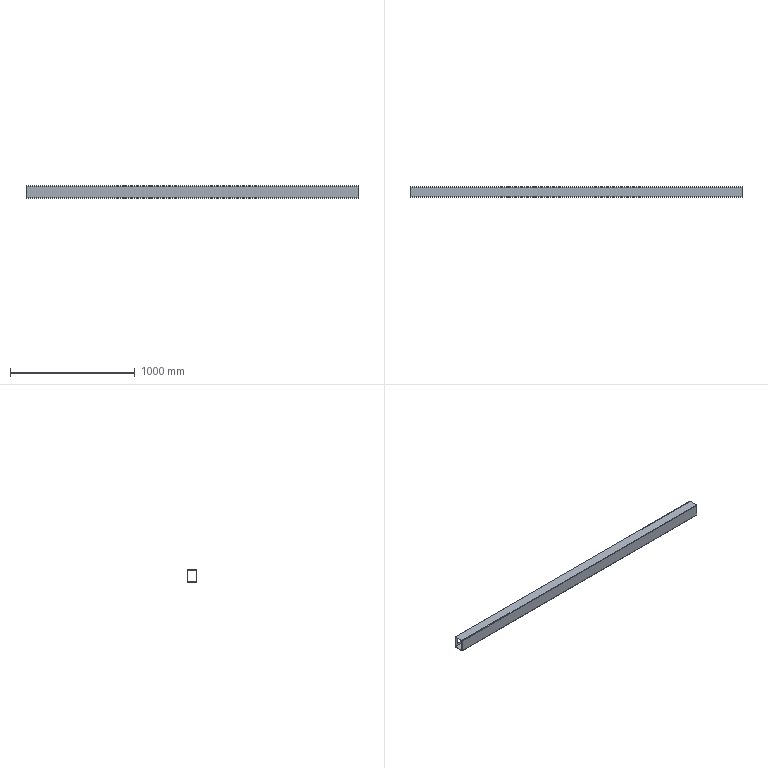Part | SolidWorks | features BaseBody 1 | 1 solid | 34 faces | box 2660 x 80 x 100 mm | volume 2713722 mm3 | plane 18 | cylinder 16 | commonest cylinder face diameters 8 x8 1 x4 7 x4
STEP:
#1=CARTESIAN_POINT('',(-1330.,40.,-46.5));
#2=VERTEX_POINT('',#1);
#3=CARTESIAN_POINT('',(-1330.,40.,46.5));
#4=VERTEX_POINT('',#3);
#5=CARTESIAN_POINT('',(-1330.,40.,46.5));
#6=DIRECTION('',(0.,0.,1.));
#7=VECTOR('',#6,1000.);
#8=LINE('',#5,#7);
#9=EDGE_CURVE('',#2,#4,#8,.T.);
#10=ORIENTED_EDGE('',*,*,#9,.T.);
#11=CARTESIAN_POINT('',(1330.,40.,46.5));
#12=VERTEX_POINT('',#11);
#13=CARTESIAN_POINT('',(1330.,40.,46.5));
#14=DIRECTION('',(-1.,0.,0.));
#15=VECTOR('',#14,1000.);
#16=LINE('',#13,#15);
#17=EDGE_CURVE('',#12,#4,#16,.T.);
#18=ORIENTED_EDGE('',*,*,#17,.F.);
#19=CARTESIAN_POINT('',(1330.,40.,-46.5));
#20=VERTEX_POINT('',#19);
#21=CARTESIAN_POINT('',(1330.,40.,46.5));
#22=DIRECTION('',(0.,0.,1.));
#23=VECTOR('',#22,1000.);
#24=LINE('',#21,#23);
#25=EDGE_CURVE('',#20,#12,#24,.T.);
#26=ORIENTED_EDGE('',*,*,#25,.F.);
#27=CARTESIAN_POINT('',(1330.,40.,-46.5));
#28=DIRECTION('',(-1.,0.,0.));
#29=VECTOR('',#28,1000.);
#30=LINE('',#27,#29);
#31=EDGE_CURVE('',#20,#2,#30,.T.);
#32=ORIENTED_EDGE('',*,*,#31,.T.);
#33=EDGE_LOOP('',(#10,#18,#26,#32));
#34=FACE_OUTER_BOUND('',#33,.T.);
#35=CARTESIAN_POINT('',(-1209.,40.,-30.));
#36=VERTEX_POINT('',#35);
#37=CARTESIAN_POINT('',(-1301.,40.,-30.));
#38=VERTEX_POINT('',#37);
#39=CARTESIAN_POINT('',(-1301.,40.,-30.));
#40=DIRECTION('',(-1.,0.,0.));
#41=VECTOR('',#40,1000.);
#42=LINE('',#39,#41);
#43=EDGE_CURVE('',#36,#38,#42,.T.);
#44=ORIENTED_EDGE('',*,*,#43,.F.);
#45=CARTESIAN_POINT('',(-1205.,40.,-26.));
#46=VERTEX_POINT('',#45);
#47=CARTESIAN_POINT('',(-1209.,40.,-26.));
#48=DIRECTION('',(0.,1.,0.));
#49=DIRECTION('',(0.,0.,1.));
#50=AXIS2_PLACEMENT_3D('',#47,#48,#49);
#51=CIRCLE('',#50,4.);
#52=EDGE_CURVE('',#46,#36,#51,.T.);
#53=ORIENTED_EDGE('',*,*,#52,.F.);
#54=CARTESIAN_POINT('',(-1205.,40.,26.));
#55=VERTEX_POINT('',#54);
#56=CARTESIAN_POINT('',(-1205.,40.,-26.));
#57=DIRECTION('',(0.,0.,-1.));
#58=VECTOR('',#57,1000.);
#59=LINE('',#56,#58);
#60=EDGE_CURVE('',#55,#46,#59,.T.);
#61=ORIENTED_EDGE('',*,*,#60,.F.);
#62=CARTESIAN_POINT('',(-1209.,40.,30.));
#63=VERTEX_POINT('',#62);
#64=CARTESIAN_POINT('',(-1209.,40.,26.));
#65=DIRECTION('',(0.,1.,0.));
#66=DIRECTION('',(0.,0.,1.));
#67=AXIS2_PLACEMENT_3D('',#64,#65,#66);
#68=CIRCLE('',#67,4.);
#69=EDGE_CURVE('',#63,#55,#68,.T.);
#70=ORIENTED_EDGE('',*,*,#69,.F.);
#71=CARTESIAN_POINT('',(-1301.,40.,30.));
#72=VERTEX_POINT('',#71);
#73=CARTESIAN_POINT('',(-1301.,40.,30.));
#74=DIRECTION('',(1.,0.,0.));
#75=VECTOR('',#74,1000.);
#76=LINE('',#73,#75);
#77=EDGE_CURVE('',#72,#63,#76,.T.);
#78=ORIENTED_EDGE('',*,*,#77,.F.);
#79=CARTESIAN_POINT('',(-1305.,40.,26.));
#80=VERTEX_POINT('',#79);
#81=CARTESIAN_POINT('',(-1301.,40.,26.));
#82=DIRECTION('',(0.,1.,0.));
#83=DIRECTION('',(0.,0.,1.));
#84=AXIS2_PLACEMENT_3D('',#81,#82,#83);
#85=CIRCLE('',#84,4.);
#86=EDGE_CURVE('',#80,#72,#85,.T.);
#87=ORIENTED_EDGE('',*,*,#86,.F.);
#88=CARTESIAN_POINT('',(-1305.,40.,-26.));
#89=VERTEX_POINT('',#88);
#90=CARTESIAN_POINT('',(-1305.,40.,-26.));
#91=DIRECTION('',(0.,0.,1.));
#92=VECTOR('',#91,1000.);
#93=LINE('',#90,#92);
#94=EDGE_CURVE('',#89,#80,#93,.T.);
#95=ORIENTED_EDGE('',*,*,#94,.F.);
#96=CARTESIAN_POINT('',(-1301.,40.,-26.));
#97=DIRECTION('',(0.,1.,0.));
#98=DIRECTION('',(0.,0.,1.));
#99=AXIS2_PLACEMENT_3D('',#96,#97,#98);
#100=CIRCLE('',#99,4.);
#101=EDGE_CURVE('',#38,#89,#100,.T.);
#102=ORIENTED_EDGE('',*,*,#101,.F.);
#103=EDGE_LOOP('',(#44,#53,#61,#70,#78,#87,#95,#102));
#104=FACE_BOUND('',#103,.T.);
#105=CARTESIAN_POINT('',(1205.,40.,-26.));
#106=VERTEX_POINT('',#105);
#107=CARTESIAN_POINT('',(1209.,40.,-30.));
#108=VERTEX_POINT('',#107);
#109=CARTESIAN_POINT('',(1209.,40.,-26.));
#110=DIRECTION('',(0.,-1.,0.));
#111=DIRECTION('',(0.,0.,1.));
#112=AXIS2_PLACEMENT_3D('',#109,#110,#111);
#113=CIRCLE('',#112,4.);
#114=EDGE_CURVE('',#106,#108,#113,.T.);
#115=ORIENTED_EDGE('',*,*,#114,.T.);
#116=CARTESIAN_POINT('',(1301.,40.,-30.));
#117=VERTEX_POINT('',#116);
#118=CARTESIAN_POINT('',(1330.,40.,-30.));
#119=DIRECTION('',(1.,0.,0.));
#120=VECTOR('',#119,1000.);
#121=LINE('',#118,#120);
#122=EDGE_CURVE('',#108,#117,#121,.T.);
#123=ORIENTED_EDGE('',*,*,#122,.T.);
#124=CARTESIAN_POINT('',(1305.,40.,-26.));
#125=VERTEX_POINT('',#124);
#126=CARTESIAN_POINT('',(1301.,40.,-26.));
#127=DIRECTION('',(0.,-1.,0.));
#128=DIRECTION('',(0.,0.,1.));
#129=AXIS2_PLACEMENT_3D('',#126,#127,#128);
#130=CIRCLE('',#129,4.);
#131=EDGE_CURVE('',#117,#125,#130,.T.);
#132=ORIENTED_EDGE('',*,*,#131,.T.);
#133=CARTESIAN_POINT('',(1305.,40.,26.));
#134=VERTEX_POINT('',#133);
#135=CARTESIAN_POINT('',(1305.,40.,46.5));
#136=DIRECTION('',(0.,0.,1.));
#137=VECTOR('',#136,1000.);
#138=LINE('',#135,#137);
#139=EDGE_CURVE('',#125,#134,#138,.T.);
#140=ORIENTED_EDGE('',*,*,#139,.T.);
#141=CARTESIAN_POINT('',(1301.,40.,30.));
#142=VERTEX_POINT('',#141);
#143=CARTESIAN_POINT('',(1301.,40.,26.));
#144=DIRECTION('',(0.,-1.,0.));
#145=DIRECTION('',(0.,0.,1.));
#146=AXIS2_PLACEMENT_3D('',#143,#144,#145);
#147=CIRCLE('',#146,4.);
#148=EDGE_CURVE('',#134,#142,#147,.T.);
#149=ORIENTED_EDGE('',*,*,#148,.T.);
#150=CARTESIAN_POINT('',(1209.,40.,30.));
#151=VERTEX_POINT('',#150);
#152=CARTESIAN_POINT('',(1330.,40.,30.));
#153=DIRECTION('',(-1.,0.,0.));
#154=VECTOR('',#153,1000.);
#155=LINE('',#152,#154);
#156=EDGE_CURVE('',#142,#151,#155,.T.);
#157=ORIENTED_EDGE('',*,*,#156,.T.);
#158=CARTESIAN_POINT('',(1205.,40.,26.));
#159=VERTEX_POINT('',#158);
#160=CARTESIAN_POINT('',(1209.,40.,26.));
#161=DIRECTION('',(0.,-1.,0.));
#162=DIRECTION('',(0.,0.,1.));
#163=AXIS2_PLACEMENT_3D('',#160,#161,#162);
#164=CIRCLE('',#163,4.);
#165=EDGE_CURVE('',#151,#159,#164,.T.);
#166=ORIENTED_EDGE('',*,*,#165,.T.);
#167=CARTESIAN_POINT('',(1205.,40.,46.5));
#168=DIRECTION('',(0.,0.,-1.));
#169=VECTOR('',#168,1000.);
#170=LINE('',#167,#169);
#171=EDGE_CURVE('',#159,#106,#170,.T.);
#172=ORIENTED_EDGE('',*,*,#171,.T.);
#173=EDGE_LOOP('',(#115,#123,#132,#140,#149,#157,#166,#172));
#174=FACE_BOUND('',#173,.T.);
#175=CARTESIAN_POINT('',(1330.,40.,46.5));
#176=DIRECTION('',(0.,-1.,0.));
#177=DIRECTION('',(0.,0.,-1.));
#178=AXIS2_PLACEMENT_3D('',#175,#176,#177);
#179=PLANE('',#178);
#180=ADVANCED_FACE('',(#34,#104,#174),#179,.F.);
#181=CARTESIAN_POINT('',(-1209.,37.,-30.));
#182=VERTEX_POINT('',#181);
#183=CARTESIAN_POINT('',(-1205.,37.,-26.));
#184=VERTEX_POINT('',#183);
#185=CARTESIAN_POINT('',(-1209.,37.,-26.));
#186=DIRECTION('',(0.,-1.,0.));
#187=DIRECTION('',(0.,0.,-1.));
#188=AXIS2_PLACEMENT_3D('',#185,#186,#187);
#189=CIRCLE('',#188,4.);
#190=EDGE_CURVE('',#182,#184,#189,.T.);
#191=ORIENTED_EDGE('',*,*,#190,.F.);
#192=CARTESIAN_POINT('',(-1301.,37.,-30.));
#193=VERTEX_POINT('',#192);
#194=CARTESIAN_POINT('',(1330.,37.,-30.));
#195=DIRECTION('',(1.,0.,0.));
#196=VECTOR('',#195,1000.);
#197=LINE('',#194,#196);
#198=EDGE_CURVE('',#193,#182,#197,.T.);
#199=ORIENTED_EDGE('',*,*,#198,.F.);
#200=CARTESIAN_POINT('',(-1305.,37.,-26.));
#201=VERTEX_POINT('',#200);
#202=CARTESIAN_POINT('',(-1301.,37.,-26.));
#203=DIRECTION('',(0.,-1.,0.));
#204=DIRECTION('',(0.,0.,-1.));
#205=AXIS2_PLACEMENT_3D('',#202,#203,#204);
#206=CIRCLE('',#205,4.);
#207=EDGE_CURVE('',#201,#193,#206,.T.);
#208=ORIENTED_EDGE('',*,*,#207,.F.);
#209=CARTESIAN_POINT('',(-1305.,37.,26.));
#210=VERTEX_POINT('',#209);
#211=CARTESIAN_POINT('',(-1305.,37.,-46.5));
#212=DIRECTION('',(0.,0.,-1.));
#213=VECTOR('',#212,1000.);
#214=LINE('',#211,#213);
#215=EDGE_CURVE('',#210,#201,#214,.T.);
#216=ORIENTED_EDGE('',*,*,#215,.F.);
#217=CARTESIAN_POINT('',(-1301.,37.,30.));
#218=VERTEX_POINT('',#217);
#219=CARTESIAN_POINT('',(-1301.,37.,26.));
#220=DIRECTION('',(0.,-1.,0.));
#221=DIRECTION('',(0.,0.,-1.));
#222=AXIS2_PLACEMENT_3D('',#219,#220,#221);
#223=CIRCLE('',#222,4.);
#224=EDGE_CURVE('',#218,#210,#223,.T.);
#225=ORIENTED_EDGE('',*,*,#224,.F.);
#226=CARTESIAN_POINT('',(-1209.,37.,30.));
#227=VERTEX_POINT('',#226);
#228=CARTESIAN_POINT('',(1330.,37.,30.));
#229=DIRECTION('',(-1.,0.,0.));
#230=VECTOR('',#229,1000.);
#231=LINE('',#228,#230);
#232=EDGE_CURVE('',#227,#218,#231,.T.);
#233=ORIENTED_EDGE('',*,*,#232,.F.);
#234=CARTESIAN_POINT('',(-1205.,37.,26.));
#235=VERTEX_POINT('',#234);
#236=CARTESIAN_POINT('',(-1209.,37.,26.));
#237=DIRECTION('',(0.,-1.,0.));
#238=DIRECTION('',(0.,0.,-1.));
#239=AXIS2_PLACEMENT_3D('',#236,#237,#238);
#240=CIRCLE('',#239,4.);
#241=EDGE_CURVE('',#235,#227,#240,.T.);
#242=ORIENTED_EDGE('',*,*,#241,.F.);
#243=CARTESIAN_POINT('',(-1205.,37.,-46.5));
#244=DIRECTION('',(0.,0.,1.));
#245=VECTOR('',#244,1000.);
#246=LINE('',#243,#245);
#247=EDGE_CURVE('',#184,#235,#246,.T.);
#248=ORIENTED_EDGE('',*,*,#247,.F.);
#249=EDGE_LOOP('',(#191,#199,#208,#216,#225,#233,#242,#248));
#250=FACE_BOUND('',#249,.T.);
#251=CARTESIAN_POINT('',(-1330.,37.,-46.5));
#252=VERTEX_POINT('',#251);
#253=CARTESIAN_POINT('',(-1330.,37.,46.5));
#254=VERTEX_POINT('',#253);
#255=CARTESIAN_POINT('',(-1330.,37.,-46.5));
#256=DIRECTION('',(0.,0.,1.));
#257=VECTOR('',#256,1000.);
#258=LINE('',#255,#257);
#259=EDGE_CURVE('',#252,#254,#258,.T.);
#260=ORIENTED_EDGE('',*,*,#259,.F.);
#261=CARTESIAN_POINT('',(1330.,37.,-46.5));
#262=VERTEX_POINT('',#261);
#263=CARTESIAN_POINT('',(1330.,37.,-46.5));
#264=DIRECTION('',(-1.,0.,0.));
#265=VECTOR('',#264,1000.);
#266=LINE('',#263,#265);
#267=EDGE_CURVE('',#262,#252,#266,.T.);
#268=ORIENTED_EDGE('',*,*,#267,.F.);
#269=CARTESIAN_POINT('',(1330.,37.,46.5));
#270=VERTEX_POINT('',#269);
#271=CARTESIAN_POINT('',(1330.,37.,-46.5));
#272=DIRECTION('',(0.,0.,1.));
#273=VECTOR('',#272,1000.);
#274=LINE('',#271,#273);
#275=EDGE_CURVE('',#262,#270,#274,.T.);
#276=ORIENTED_EDGE('',*,*,#275,.T.);
#277=CARTESIAN_POINT('',(1330.,37.,46.5));
#278=DIRECTION('',(-1.,0.,0.));
#279=VECTOR('',#278,1000.);
#280=LINE('',#277,#279);
#281=EDGE_CURVE('',#270,#254,#280,.T.);
#282=ORIENTED_EDGE('',*,*,#281,.T.);
#283=EDGE_LOOP('',(#260,#268,#276,#282));
#284=FACE_OUTER_BOUND('',#283,.T.);
#285=CARTESIAN_POINT('',(1301.,37.,-30.));
#286=VERTEX_POINT('',#285);
#287=CARTESIAN_POINT('',(1209.,37.,-30.));
#288=VERTEX_POINT('',#287);
#289=CARTESIAN_POINT('',(1330.,37.,-30.));
#290=DIRECTION('',(-1.,0.,0.));
#291=VECTOR('',#290,1000.);
#292=LINE('',#289,#291);
#293=EDGE_CURVE('',#286,#288,#292,.T.);
#294=ORIENTED_EDGE('',*,*,#293,.T.);
#295=CARTESIAN_POINT('',(1205.,37.,-26.));
#296=VERTEX_POINT('',#295);
#297=CARTESIAN_POINT('',(1209.,37.,-26.));
#298=DIRECTION('',(0.,1.,0.));
#299=DIRECTION('',(0.,0.,-1.));
#300=AXIS2_PLACEMENT_3D('',#297,#298,#299);
#301=CIRCLE('',#300,4.);
#302=EDGE_CURVE('',#288,#296,#301,.T.);
#303=ORIENTED_EDGE('',*,*,#302,.T.);
#304=CARTESIAN_POINT('',(1205.,37.,26.));
#305=VERTEX_POINT('',#304);
#306=CARTESIAN_POINT('',(1205.,37.,-46.5));
#307=DIRECTION('',(0.,0.,1.));
#308=VECTOR('',#307,1000.);
#309=LINE('',#306,#308);
#310=EDGE_CURVE('',#296,#305,#309,.T.);
#311=ORIENTED_EDGE('',*,*,#310,.T.);
#312=CARTESIAN_POINT('',(1209.,37.,30.));
#313=VERTEX_POINT('',#312);
#314=CARTESIAN_POINT('',(1209.,37.,26.));
#315=DIRECTION('',(0.,1.,0.));
#316=DIRECTION('',(0.,0.,-1.));
#317=AXIS2_PLACEMENT_3D('',#314,#315,#316);
#318=CIRCLE('',#317,4.);
#319=EDGE_CURVE('',#305,#313,#318,.T.);
#320=ORIENTED_EDGE('',*,*,#319,.T.);
#321=CARTESIAN_POINT('',(1301.,37.,30.));
#322=VERTEX_POINT('',#321);
#323=CARTESIAN_POINT('',(1330.,37.,30.));
#324=DIRECTION('',(1.,0.,0.));
#325=VECTOR('',#324,1000.);
#326=LINE('',#323,#325);
#327=EDGE_CURVE('',#313,#322,#326,.T.);
#328=ORIENTED_EDGE('',*,*,#327,.T.);
#329=CARTESIAN_POINT('',(1305.,37.,26.));
#330=VERTEX_POINT('',#329);
#331=CARTESIAN_POINT('',(1301.,37.,26.));
#332=DIRECTION('',(0.,1.,0.));
#333=DIRECTION('',(0.,0.,-1.));
#334=AXIS2_PLACEMENT_3D('',#331,#332,#333);
#335=CIRCLE('',#334,4.);
#336=EDGE_CURVE('',#322,#330,#335,.T.);
#337=ORIENTED_EDGE('',*,*,#336,.T.);
#338=CARTESIAN_POINT('',(1305.,37.,-26.));
#339=VERTEX_POINT('',#338);
#340=CARTESIAN_POINT('',(1305.,37.,-46.5));
#341=DIRECTION('',(0.,0.,-1.));
#342=VECTOR('',#341,1000.);
#343=LINE('',#340,#342);
#344=EDGE_CURVE('',#330,#339,#343,.T.);
#345=ORIENTED_EDGE('',*,*,#344,.T.);
#346=CARTESIAN_POINT('',(1301.,37.,-26.));
#347=DIRECTION('',(0.,1.,0.));
#348=DIRECTION('',(0.,0.,-1.));
#349=AXIS2_PLACEMENT_3D('',#346,#347,#348);
#350=CIRCLE('',#349,4.);
#351=EDGE_CURVE('',#339,#286,#350,.T.);
#352=ORIENTED_EDGE('',*,*,#351,.T.);
#353=EDGE_LOOP('',(#294,#303,#311,#320,#328,#337,#345,#352));
#354=FACE_BOUND('',#353,.T.);
#355=CARTESIAN_POINT('',(1330.,37.,-46.5));
#356=DIRECTION('',(0.,-1.,0.));
#357=DIRECTION('',(0.,0.,-1.));
#358=AXIS2_PLACEMENT_3D('',#355,#356,#357);
#359=PLANE('',#358);
#360=ADVANCED_FACE('',(#250,#284,#354),#359,.T.);
#361=CARTESIAN_POINT('',(1330.,36.5,-50.));
#362=VERTEX_POINT('',#361);
#363=CARTESIAN_POINT('',(1330.,36.5,-46.5));
#364=DIRECTION('',(1.,0.,0.));
#365=DIRECTION('',(0.,0.,1.));
#366=AXIS2_PLACEMENT_3D('',#363,#364,#365);
#367=CIRCLE('',#366,3.5);
#368=EDGE_CURVE('',#362,#20,#367,.T.);
#369=ORIENTED_EDGE('',*,*,#368,.T.);
#370=ORIENTED_EDGE('',*,*,#25,.T.);
#371=CARTESIAN_POINT('',(1330.,36.5,50.));
#372=VERTEX_POINT('',#371);
#373=CARTESIAN_POINT('',(1330.,36.5,46.5));
#374=DIRECTION('',(1.,0.,0.));
#375=DIRECTION('',(0.,0.,-1.));
#376=AXIS2_PLACEMENT_3D('',#373,#374,#375);
#377=CIRCLE('',#376,3.5);
#378=EDGE_CURVE('',#12,#372,#377,.T.);
#379=ORIENTED_EDGE('',*,*,#378,.T.);
#380=CARTESIAN_POINT('',(1330.,-36.5,50.));
#381=VERTEX_POINT('',#380);
#382=CARTESIAN_POINT('',(1330.,36.5,50.));
#383=DIRECTION('',(0.,-1.,0.));
#384=VECTOR('',#383,1000.);
#385=LINE('',#382,#384);
#386=EDGE_CURVE('',#372,#381,#385,.T.);
#387=ORIENTED_EDGE('',*,*,#386,.T.);
#388=CARTESIAN_POINT('',(1330.,-40.,46.5));
#389=VERTEX_POINT('',#388);
#390=CARTESIAN_POINT('',(1330.,-36.5,46.5));
#391=DIRECTION('',(1.,0.,0.));
#392=DIRECTION('',(0.,0.,-1.));
#393=AXIS2_PLACEMENT_3D('',#390,#391,#392);
#394=CIRCLE('',#393,3.5);
#395=EDGE_CURVE('',#381,#389,#394,.T.);
#396=ORIENTED_EDGE('',*,*,#395,.T.);
#397=CARTESIAN_POINT('',(1330.,-40.,-46.5));
#398=VERTEX_POINT('',#397);
#399=CARTESIAN_POINT('',(1330.,-40.,46.5));
#400=DIRECTION('',(0.,0.,-1.));
#401=VECTOR('',#400,1000.);
#402=LINE('',#399,#401);
#403=EDGE_CURVE('',#389,#398,#402,.T.);
#404=ORIENTED_EDGE('',*,*,#403,.T.);
#405=CARTESIAN_POINT('',(1330.,-36.5,-50.));
#406=VERTEX_POINT('',#405);
#407=CARTESIAN_POINT('',(1330.,-36.5,-46.5));
#408=DIRECTION('',(1.,0.,0.));
#409=DIRECTION('',(0.,0.,-1.));
#410=AXIS2_PLACEMENT_3D('',#407,#408,#409);
#411=CIRCLE('',#410,3.5);
#412=EDGE_CURVE('',#398,#406,#411,.T.);
#413=ORIENTED_EDGE('',*,*,#412,.T.);
#414=CARTESIAN_POINT('',(1330.,36.5,-50.));
#415=DIRECTION('',(0.,1.,0.));
#416=VECTOR('',#415,1000.);
#417=LINE('',#414,#416);
#418=EDGE_CURVE('',#406,#362,#417,.T.);
#419=ORIENTED_EDGE('',*,*,#418,.T.);
#420=EDGE_LOOP('',(#369,#370,#379,#387,#396,#404,#413,#419));
#421=FACE_OUTER_BOUND('',#420,.T.);
#422=ORIENTED_EDGE('',*,*,#275,.F.);
#423=CARTESIAN_POINT('',(1330.,36.5,-47.));
#424=VERTEX_POINT('',#423);
#425=CARTESIAN_POINT('',(1330.,36.5,-46.5));
#426=DIRECTION('',(1.,0.,0.));
#427=DIRECTION('',(0.,0.,1.));
#428=AXIS2_PLACEMENT_3D('',#425,#426,#427);
#429=CIRCLE('',#428,0.5);
#430=EDGE_CURVE('',#424,#262,#429,.T.);
#431=ORIENTED_EDGE('',*,*,#430,.F.);
#432=CARTESIAN_POINT('',(1330.,-36.5,-47.));
#433=VERTEX_POINT('',#432);
#434=CARTESIAN_POINT('',(1330.,36.5,-47.));
#435=DIRECTION('',(0.,1.,0.));
#436=VECTOR('',#435,1000.);
#437=LINE('',#434,#436);
#438=EDGE_CURVE('',#433,#424,#437,.T.);
#439=ORIENTED_EDGE('',*,*,#438,.F.);
#440=CARTESIAN_POINT('',(1330.,-37.,-46.5));
#441=VERTEX_POINT('',#440);
#442=CARTESIAN_POINT('',(1330.,-36.5,-46.5));
#443=DIRECTION('',(1.,0.,0.));
#444=DIRECTION('',(0.,0.,1.));
#445=AXIS2_PLACEMENT_3D('',#442,#443,#444);
#446=CIRCLE('',#445,0.5);
#447=EDGE_CURVE('',#441,#433,#446,.T.);
#448=ORIENTED_EDGE('',*,*,#447,.F.);
#449=CARTESIAN_POINT('',(1330.,-37.,46.5));
#450=VERTEX_POINT('',#449);
#451=CARTESIAN_POINT('',(1330.,-37.,-46.5));
#452=DIRECTION('',(0.,0.,-1.));
#453=VECTOR('',#452,1000.);
#454=LINE('',#451,#453);
#455=EDGE_CURVE('',#450,#441,#454,.T.);
#456=ORIENTED_EDGE('',*,*,#455,.F.);
#457=CARTESIAN_POINT('',(1330.,-36.5,47.));
#458=VERTEX_POINT('',#457);
#459=CARTESIAN_POINT('',(1330.,-36.5,46.5));
#460=DIRECTION('',(1.,0.,0.));
#461=DIRECTION('',(0.,0.,1.));
#462=AXIS2_PLACEMENT_3D('',#459,#460,#461);
#463=CIRCLE('',#462,0.5);
#464=EDGE_CURVE('',#458,#450,#463,.T.);
#465=ORIENTED_EDGE('',*,*,#464,.F.);
#466=CARTESIAN_POINT('',(1330.,36.5,47.));
#467=VERTEX_POINT('',#466);
#468=CARTESIAN_POINT('',(1330.,36.5,47.));
#469=DIRECTION('',(0.,-1.,0.));
#470=VECTOR('',#469,1000.);
#471=LINE('',#468,#470);
#472=EDGE_CURVE('',#467,#458,#471,.T.);
#473=ORIENTED_EDGE('',*,*,#472,.F.);
#474=CARTESIAN_POINT('',(1330.,36.5,46.5));
#475=DIRECTION('',(1.,0.,0.));
#476=DIRECTION('',(0.,0.,1.));
#477=AXIS2_PLACEMENT_3D('',#474,#475,#476);
#478=CIRCLE('',#477,0.5);
#479=EDGE_CURVE('',#270,#467,#478,.T.);
#480=ORIENTED_EDGE('',*,*,#479,.F.);
#481=EDGE_LOOP('',(#422,#431,#439,#448,#456,#465,#473,#480));
#482=FACE_BOUND('',#481,.T.);
#483=CARTESIAN_POINT('',(1330.,36.5,-46.5));
#484=DIRECTION('',(1.,0.,0.));
#485=DIRECTION('',(0.,0.,-1.));
#486=AXIS2_PLACEMENT_3D('',#483,#484,#485);
#487=PLANE('',#486);
#488=ADVANCED_FACE('',(#421,#482),#487,.T.);
#489=CARTESIAN_POINT('',(-1330.,36.5,-50.));
#490=VERTEX_POINT('',#489);
#491=CARTESIAN_POINT('',(-1330.,36.5,-46.5));
#492=DIRECTION('',(1.,0.,0.));
#493=DIRECTION('',(0.,0.,1.));
#494=AXIS2_PLACEMENT_3D('',#491,#492,#493);
#495=CIRCLE('',#494,3.5);
#496=EDGE_CURVE('',#490,#2,#495,.T.);
#497=ORIENTED_EDGE('',*,*,#496,.F.);
#498=CARTESIAN_POINT('',(-1330.,-36.5,-50.));
#499=VERTEX_POINT('',#498);
#500=CARTESIAN_POINT('',(-1330.,36.5,-50.));
#501=DIRECTION('',(0.,1.,0.));
#502=VECTOR('',#501,1000.);
#503=LINE('',#500,#502);
#504=EDGE_CURVE('',#499,#490,#503,.T.);
#505=ORIENTED_EDGE('',*,*,#504,.F.);
#506=CARTESIAN_POINT('',(-1330.,-40.,-46.5));
#507=VERTEX_POINT('',#506);
#508=CARTESIAN_POINT('',(-1330.,-36.5,-46.5));
#509=DIRECTION('',(1.,0.,0.));
#510=DIRECTION('',(0.,0.,-1.));
#511=AXIS2_PLACEMENT_3D('',#508,#509,#510);
#512=CIRCLE('',#511,3.5);
#513=EDGE_CURVE('',#507,#499,#512,.T.);
#514=ORIENTED_EDGE('',*,*,#513,.F.);
#515=CARTESIAN_POINT('',(-1330.,-40.,46.5));
#516=VERTEX_POINT('',#515);
#517=CARTESIAN_POINT('',(-1330.,-40.,46.5));
#518=DIRECTION('',(0.,0.,-1.));
#519=VECTOR('',#518,1000.);
#520=LINE('',#517,#519);
#521=EDGE_CURVE('',#516,#507,#520,.T.);
#522=ORIENTED_EDGE('',*,*,#521,.F.);
#523=CARTESIAN_POINT('',(-1330.,-36.5,50.));
#524=VERTEX_POINT('',#523);
#525=CARTESIAN_POINT('',(-1330.,-36.5,46.5));
#526=DIRECTION('',(1.,0.,0.));
#527=DIRECTION('',(0.,0.,-1.));
#528=AXIS2_PLACEMENT_3D('',#525,#526,#527);
#529=CIRCLE('',#528,3.5);
#530=EDGE_CURVE('',#524,#516,#529,.T.);
#531=ORIENTED_EDGE('',*,*,#530,.F.);
#532=CARTESIAN_POINT('',(-1330.,36.5,50.));
#533=VERTEX_POINT('',#532);
#534=CARTESIAN_POINT('',(-1330.,36.5,50.));
#535=DIRECTION('',(0.,-1.,0.));
#536=VECTOR('',#535,1000.);
#537=LINE('',#534,#536);
#538=EDGE_CURVE('',#533,#524,#537,.T.);
#539=ORIENTED_EDGE('',*,*,#538,.F.);
#540=CARTESIAN_POINT('',(-1330.,36.5,46.5));
#541=DIRECTION('',(1.,0.,0.));
#542=DIRECTION('',(0.,0.,-1.));
#543=AXIS2_PLACEMENT_3D('',#540,#541,#542);
#544=CIRCLE('',#543,3.5);
#545=EDGE_CURVE('',#4,#533,#544,.T.);
#546=ORIENTED_EDGE('',*,*,#545,.F.);
#547=ORIENTED_EDGE('',*,*,#9,.F.);
#548=EDGE_LOOP('',(#497,#505,#514,#522,#531,#539,#546,#547));
#549=FACE_OUTER_BOUND('',#548,.T.);
#550=CARTESIAN_POINT('',(-1330.,36.5,-47.));
#551=VERTEX_POINT('',#550);
#552=CARTESIAN_POINT('',(-1330.,36.5,-46.5));
#553=DIRECTION('',(1.,0.,0.));
#554=DIRECTION('',(0.,0.,1.));
#555=AXIS2_PLACEMENT_3D('',#552,#553,#554);
#556=CIRCLE('',#555,0.5);
#557=EDGE_CURVE('',#551,#252,#556,.T.);
#558=ORIENTED_EDGE('',*,*,#557,.T.);
#559=ORIENTED_EDGE('',*,*,#259,.T.);
#560=CARTESIAN_POINT('',(-1330.,36.5,47.));
#561=VERTEX_POINT('',#560);
#562=CARTESIAN_POINT('',(-1330.,36.5,46.5));
#563=DIRECTION('',(1.,0.,0.));
#564=DIRECTION('',(0.,0.,1.));
#565=AXIS2_PLACEMENT_3D('',#562,#563,#564);
#566=CIRCLE('',#565,0.5);
#567=EDGE_CURVE('',#254,#561,#566,.T.);
#568=ORIENTED_EDGE('',*,*,#567,.T.);
#569=CARTESIAN_POINT('',(-1330.,-36.5,47.));
#570=VERTEX_POINT('',#569);
#571=CARTESIAN_POINT('',(-1330.,36.5,47.));
#572=DIRECTION('',(0.,-1.,0.));
#573=VECTOR('',#572,1000.);
#574=LINE('',#571,#573);
#575=EDGE_CURVE('',#561,#570,#574,.T.);
#576=ORIENTED_EDGE('',*,*,#575,.T.);
#577=CARTESIAN_POINT('',(-1330.,-37.,46.5));
#578=VERTEX_POINT('',#577);
#579=CARTESIAN_POINT('',(-1330.,-36.5,46.5));
#580=DIRECTION('',(1.,0.,0.));
#581=DIRECTION('',(0.,0.,1.));
#582=AXIS2_PLACEMENT_3D('',#579,#580,#581);
#583=CIRCLE('',#582,0.5);
#584=EDGE_CURVE('',#570,#578,#583,.T.);
#585=ORIENTED_EDGE('',*,*,#584,.T.);
#586=CARTESIAN_POINT('',(-1330.,-37.,-46.5));
#587=VERTEX_POINT('',#586);
#588=CARTESIAN_POINT('',(-1330.,-37.,-46.5));
#589=DIRECTION('',(0.,0.,-1.));
#590=VECTOR('',#589,1000.);
#591=LINE('',#588,#590);
#592=EDGE_CURVE('',#578,#587,#591,.T.);
#593=ORIENTED_EDGE('',*,*,#592,.T.);
#594=CARTESIAN_POINT('',(-1330.,-36.5,-47.));
#595=VERTEX_POINT('',#594);
#596=CARTESIAN_POINT('',(-1330.,-36.5,-46.5));
#597=DIRECTION('',(1.,0.,0.));
#598=DIRECTION('',(0.,0.,1.));
#599=AXIS2_PLACEMENT_3D('',#596,#597,#598);
#600=CIRCLE('',#599,0.5);
#601=EDGE_CURVE('',#587,#595,#600,.T.);
#602=ORIENTED_EDGE('',*,*,#601,.T.);
#603=CARTESIAN_POINT('',(-1330.,36.5,-47.));
#604=DIRECTION('',(0.,1.,0.));
#605=VECTOR('',#604,1000.);
#606=LINE('',#603,#605);
#607=EDGE_CURVE('',#595,#551,#606,.T.);
#608=ORIENTED_EDGE('',*,*,#607,.T.);
#609=EDGE_LOOP('',(#558,#559,#568,#576,#585,#593,#602,#608));
#610=FACE_BOUND('',#609,.T.);
#611=CARTESIAN_POINT('',(-1330.,36.5,-46.5));
#612=DIRECTION('',(1.,0.,0.));
#613=DIRECTION('',(0.,0.,-1.));
#614=AXIS2_PLACEMENT_3D('',#611,#612,#613);
#615=PLANE('',#614);
#616=ADVANCED_FACE('',(#549,#610),#615,.F.);
#617=ORIENTED_EDGE('',*,*,#496,.T.);
#618=ORIENTED_EDGE('',*,*,#31,.F.);
#619=ORIENTED_EDGE('',*,*,#368,.F.);
#620=CARTESIAN_POINT('',(1330.,36.5,-50.));
#621=DIRECTION('',(-1.,0.,0.));
#622=VECTOR('',#621,1000.);
#623=LINE('',#620,#622);
#624=EDGE_CURVE('',#362,#490,#623,.T.);
#625=ORIENTED_EDGE('',*,*,#624,.T.);
#626=EDGE_LOOP('',(#617,#618,#619,#625));
#627=FACE_OUTER_BOUND('',#626,.T.);
#628=CARTESIAN_POINT('',(1330.,36.5,-46.5));
#629=DIRECTION('',(-1.,0.,0.));
#630=DIRECTION('',(0.,0.,1.));
#631=AXIS2_PLACEMENT_3D('',#628,#629,#630);
#632=CYLINDRICAL_SURFACE('',#631,3.5);
#633=ADVANCED_FACE('',(#627),#632,.T.);
#634=ORIENTED_EDGE('',*,*,#545,.T.);
#635=CARTESIAN_POINT('',(1330.,36.5,50.));
#636=DIRECTION('',(-1.,0.,0.));
#637=VECTOR('',#636,1000.);
#638=LINE('',#635,#637);
#639=EDGE_CURVE('',#372,#533,#638,.T.);
#640=ORIENTED_EDGE('',*,*,#639,.F.);
#641=ORIENTED_EDGE('',*,*,#378,.F.);
#642=ORIENTED_EDGE('',*,*,#17,.T.);
#643=EDGE_LOOP('',(#634,#640,#641,#642));
#644=FACE_OUTER_BOUND('',#643,.T.);
#645=CARTESIAN_POINT('',(1330.,36.5,46.5));
#646=DIRECTION('',(-1.,0.,0.));
#647=DIRECTION('',(0.,0.,1.));
#648=AXIS2_PLACEMENT_3D('',#645,#646,#647);
#649=CYLINDRICAL_SURFACE('',#648,3.5);
#650=ADVANCED_FACE('',(#644),#649,.T.);
#651=ORIENTED_EDGE('',*,*,#538,.T.);
#652=CARTESIAN_POINT('',(1330.,-36.5,50.));
#653=DIRECTION('',(-1.,0.,0.));
#654=VECTOR('',#653,1000.);
#655=LINE('',#652,#654);
#656=EDGE_CURVE('',#381,#524,#655,.T.);
#657=ORIENTED_EDGE('',*,*,#656,.F.);
#658=ORIENTED_EDGE('',*,*,#386,.F.);
#659=ORIENTED_EDGE('',*,*,#639,.T.);
#660=EDGE_LOOP('',(#651,#657,#658,#659));
#661=FACE_OUTER_BOUND('',#660,.T.);
#662=CARTESIAN_POINT('',(1330.,36.5,50.));
#663=DIRECTION('',(0.,0.,-1.));
#664=DIRECTION('',(0.,1.,0.));
#665=AXIS2_PLACEMENT_3D('',#662,#663,#664);
#666=PLANE('',#665);
#667=ADVANCED_FACE('',(#661),#666,.F.);
#668=ORIENTED_EDGE('',*,*,#530,.T.);
#669=CARTESIAN_POINT('',(1330.,-40.,46.5));
#670=DIRECTION('',(-1.,0.,0.));
#671=VECTOR('',#670,1000.);
#672=LINE('',#669,#671);
#673=EDGE_CURVE('',#389,#516,#672,.T.);
#674=ORIENTED_EDGE('',*,*,#673,.F.);
#675=ORIENTED_EDGE('',*,*,#395,.F.);
#676=ORIENTED_EDGE('',*,*,#656,.T.);
#677=EDGE_LOOP('',(#668,#674,#675,#676));
#678=FACE_OUTER_BOUND('',#677,.T.);
#679=CARTESIAN_POINT('',(1330.,-36.5,46.5));
#680=DIRECTION('',(-1.,0.,0.));
#681=DIRECTION('',(0.,0.,1.));
#682=AXIS2_PLACEMENT_3D('',#679,#680,#681);
#683=CYLINDRICAL_SURFACE('',#682,3.5);
#684=ADVANCED_FACE('',(#678),#683,.T.);
#685=ORIENTED_EDGE('',*,*,#521,.T.);
#686=CARTESIAN_POINT('',(1330.,-40.,-46.5));
#687=DIRECTION('',(-1.,0.,0.));
#688=VECTOR('',#687,1000.);
#689=LINE('',#686,#688);
#690=EDGE_CURVE('',#398,#507,#689,.T.);
#691=ORIENTED_EDGE('',*,*,#690,.F.);
#692=ORIENTED_EDGE('',*,*,#403,.F.);
#693=ORIENTED_EDGE('',*,*,#673,.T.);
#694=EDGE_LOOP('',(#685,#691,#692,#693));
#695=FACE_OUTER_BOUND('',#694,.T.);
#696=CARTESIAN_POINT('',(1330.,-40.,46.5));
#697=DIRECTION('',(0.,1.,0.));
#698=DIRECTION('',(0.,0.,1.));
#699=AXIS2_PLACEMENT_3D('',#696,#697,#698);
#700=PLANE('',#699);
#701=ADVANCED_FACE('',(#695),#700,.F.);
#702=ORIENTED_EDGE('',*,*,#513,.T.);
#703=CARTESIAN_POINT('',(1330.,-36.5,-50.));
#704=DIRECTION('',(-1.,0.,0.));
#705=VECTOR('',#704,1000.);
#706=LINE('',#703,#705);
#707=EDGE_CURVE('',#406,#499,#706,.T.);
#708=ORIENTED_EDGE('',*,*,#707,.F.);
#709=ORIENTED_EDGE('',*,*,#412,.F.);
#710=ORIENTED_EDGE('',*,*,#690,.T.);
#711=EDGE_LOOP('',(#702,#708,#709,#710));
#712=FACE_OUTER_BOUND('',#711,.T.);
#713=CARTESIAN_POINT('',(1330.,-36.5,-46.5));
#714=DIRECTION('',(-1.,0.,0.));
#715=DIRECTION('',(0.,0.,1.));
#716=AXIS2_PLACEMENT_3D('',#713,#714,#715);
#717=CYLINDRICAL_SURFACE('',#716,3.5);
#718=ADVANCED_FACE('',(#712),#717,.T.);
#719=ORIENTED_EDGE('',*,*,#504,.T.);
#720=ORIENTED_EDGE('',*,*,#624,.F.);
#721=ORIENTED_EDGE('',*,*,#418,.F.);
#722=ORIENTED_EDGE('',*,*,#707,.T.);
#723=EDGE_LOOP('',(#719,#720,#721,#722));
#724=FACE_OUTER_BOUND('',#723,.T.);
#725=CARTESIAN_POINT('',(1330.,36.5,-50.));
#726=DIRECTION('',(0.,0.,1.));
#727=DIRECTION('',(0.,-1.,0.));
#728=AXIS2_PLACEMENT_3D('',#725,#726,#727);
#729=PLANE('',#728);
#730=ADVANCED_FACE('',(#724),#729,.F.);
#731=ORIENTED_EDGE('',*,*,#557,.F.);
#732=CARTESIAN_POINT('',(1330.,36.5,-47.));
#733=DIRECTION('',(-1.,0.,0.));
#734=VECTOR('',#733,1000.);
#735=LINE('',#732,#734);
#736=EDGE_CURVE('',#424,#551,#735,.T.);
#737=ORIENTED_EDGE('',*,*,#736,.F.);
#738=ORIENTED_EDGE('',*,*,#430,.T.);
#739=ORIENTED_EDGE('',*,*,#267,.T.);
#740=EDGE_LOOP('',(#731,#737,#738,#739));
#741=FACE_OUTER_BOUND('',#740,.T.);
#742=CARTESIAN_POINT('',(1330.,36.5,-46.5));
#743=DIRECTION('',(-1.,0.,0.));
#744=DIRECTION('',(0.,0.,1.));
#745=AXIS2_PLACEMENT_3D('',#742,#743,#744);
#746=CYLINDRICAL_SURFACE('',#745,0.5);
#747=ADVANCED_FACE('',(#741),#746,.F.);
#748=ORIENTED_EDGE('',*,*,#567,.F.);
#749=ORIENTED_EDGE('',*,*,#281,.F.);
#750=ORIENTED_EDGE('',*,*,#479,.T.);
#751=CARTESIAN_POINT('',(1330.,36.5,47.));
#752=DIRECTION('',(-1.,0.,0.));
#753=VECTOR('',#752,1000.);
#754=LINE('',#751,#753);
#755=EDGE_CURVE('',#467,#561,#754,.T.);
#756=ORIENTED_EDGE('',*,*,#755,.T.);
#757=EDGE_LOOP('',(#748,#749,#750,#756));
#758=FACE_OUTER_BOUND('',#757,.T.);
#759=CARTESIAN_POINT('',(1330.,36.5,46.5));
#760=DIRECTION('',(-1.,0.,0.));
#761=DIRECTION('',(0.,0.,1.));
#762=AXIS2_PLACEMENT_3D('',#759,#760,#761);
#763=CYLINDRICAL_SURFACE('',#762,0.5);
#764=ADVANCED_FACE('',(#758),#763,.F.);
#765=ORIENTED_EDGE('',*,*,#575,.F.);
#766=ORIENTED_EDGE('',*,*,#755,.F.);
#767=ORIENTED_EDGE('',*,*,#472,.T.);
#768=CARTESIAN_POINT('',(1330.,-36.5,47.));
#769=DIRECTION('',(-1.,0.,0.));
#770=VECTOR('',#769,1000.);
#771=LINE('',#768,#770);
#772=EDGE_CURVE('',#458,#570,#771,.T.);
#773=ORIENTED_EDGE('',*,*,#772,.T.);
#774=EDGE_LOOP('',(#765,#766,#767,#773));
#775=FACE_OUTER_BOUND('',#774,.T.);
#776=CARTESIAN_POINT('',(1330.,36.5,47.));
#777=DIRECTION('',(0.,0.,-1.));
#778=DIRECTION('',(0.,1.,0.));
#779=AXIS2_PLACEMENT_3D('',#776,#777,#778);
#780=PLANE('',#779);
#781=ADVANCED_FACE('',(#775),#780,.T.);
#782=ORIENTED_EDGE('',*,*,#584,.F.);
#783=ORIENTED_EDGE('',*,*,#772,.F.);
#784=ORIENTED_EDGE('',*,*,#464,.T.);
#785=CARTESIAN_POINT('',(1330.,-37.,46.5));
#786=DIRECTION('',(-1.,0.,0.));
#787=VECTOR('',#786,1000.);
#788=LINE('',#785,#787);
#789=EDGE_CURVE('',#450,#578,#788,.T.);
#790=ORIENTED_EDGE('',*,*,#789,.T.);
#791=EDGE_LOOP('',(#782,#783,#784,#790));
#792=FACE_OUTER_BOUND('',#791,.T.);
#793=CARTESIAN_POINT('',(1330.,-36.5,46.5));
#794=DIRECTION('',(-1.,0.,0.));
#795=DIRECTION('',(0.,0.,1.));
#796=AXIS2_PLACEMENT_3D('',#793,#794,#795);
#797=CYLINDRICAL_SURFACE('',#796,0.5);
#798=ADVANCED_FACE('',(#792),#797,.F.);
#799=ORIENTED_EDGE('',*,*,#592,.F.);
#800=ORIENTED_EDGE('',*,*,#789,.F.);
#801=ORIENTED_EDGE('',*,*,#455,.T.);
#802=CARTESIAN_POINT('',(1330.,-37.,-46.5));
#803=DIRECTION('',(-1.,0.,0.));
#804=VECTOR('',#803,1000.);
#805=LINE('',#802,#804);
#806=EDGE_CURVE('',#441,#587,#805,.T.);
#807=ORIENTED_EDGE('',*,*,#806,.T.);
#808=EDGE_LOOP('',(#799,#800,#801,#807));
#809=FACE_OUTER_BOUND('',#808,.T.);
#810=CARTESIAN_POINT('',(1330.,-37.,-46.5));
#811=DIRECTION('',(0.,1.,0.));
#812=DIRECTION('',(0.,0.,1.));
#813=AXIS2_PLACEMENT_3D('',#810,#811,#812);
#814=PLANE('',#813);
#815=ADVANCED_FACE('',(#809),#814,.T.);
#816=ORIENTED_EDGE('',*,*,#601,.F.);
#817=ORIENTED_EDGE('',*,*,#806,.F.);
#818=ORIENTED_EDGE('',*,*,#447,.T.);
#819=CARTESIAN_POINT('',(1330.,-36.5,-47.));
#820=DIRECTION('',(-1.,0.,0.));
#821=VECTOR('',#820,1000.);
#822=LINE('',#819,#821);
#823=EDGE_CURVE('',#433,#595,#822,.T.);
#824=ORIENTED_EDGE('',*,*,#823,.T.);
#825=EDGE_LOOP('',(#816,#817,#818,#824));
#826=FACE_OUTER_BOUND('',#825,.T.);
#827=CARTESIAN_POINT('',(1330.,-36.5,-46.5));
#828=DIRECTION('',(-1.,0.,0.));
#829=DIRECTION('',(0.,0.,1.));
#830=AXIS2_PLACEMENT_3D('',#827,#828,#829);
#831=CYLINDRICAL_SURFACE('',#830,0.5);
#832=ADVANCED_FACE('',(#826),#831,.F.);
#833=ORIENTED_EDGE('',*,*,#607,.F.);
#834=ORIENTED_EDGE('',*,*,#823,.F.);
#835=ORIENTED_EDGE('',*,*,#438,.T.);
#836=ORIENTED_EDGE('',*,*,#736,.T.);
#837=EDGE_LOOP('',(#833,#834,#835,#836));
#838=FACE_OUTER_BOUND('',#837,.T.);
#839=CARTESIAN_POINT('',(1330.,36.5,-47.));
#840=DIRECTION('',(0.,0.,1.));
#841=DIRECTION('',(0.,-1.,0.));
#842=AXIS2_PLACEMENT_3D('',#839,#840,#841);
#843=PLANE('',#842);
#844=ADVANCED_FACE('',(#838),#843,.T.);
#845=CARTESIAN_POINT('',(-1209.,30.,-30.));
#846=DIRECTION('',(0.,1.,0.));
#847=VECTOR('',#846,1000.);
#848=LINE('',#845,#847);
#849=EDGE_CURVE('',#182,#36,#848,.T.);
#850=ORIENTED_EDGE('',*,*,#849,.F.);
#851=ORIENTED_EDGE('',*,*,#190,.T.);
#852=CARTESIAN_POINT('',(-1205.,30.,-26.));
#853=DIRECTION('',(0.,1.,0.));
#854=VECTOR('',#853,1000.);
#855=LINE('',#852,#854);
#856=EDGE_CURVE('',#184,#46,#855,.T.);
#857=ORIENTED_EDGE('',*,*,#856,.T.);
#858=ORIENTED_EDGE('',*,*,#52,.T.);
#859=EDGE_LOOP('',(#850,#851,#857,#858));
#860=FACE_OUTER_BOUND('',#859,.T.);
#861=CARTESIAN_POINT('',(-1209.,30.,-26.));
#862=DIRECTION('',(0.,1.,0.));
#863=DIRECTION('',(0.,0.,1.));
#864=AXIS2_PLACEMENT_3D('',#861,#862,#863);
#865=CYLINDRICAL_SURFACE('',#864,4.);
#866=ADVANCED_FACE('',(#860),#865,.F.);
#867=ORIENTED_EDGE('',*,*,#856,.F.);
#868=ORIENTED_EDGE('',*,*,#247,.T.);
#869=CARTESIAN_POINT('',(-1205.,30.,26.));
#870=DIRECTION('',(0.,1.,0.));
#871=VECTOR('',#870,1000.);
#872=LINE('',#869,#871);
#873=EDGE_CURVE('',#235,#55,#872,.T.);
#874=ORIENTED_EDGE('',*,*,#873,.T.);
#875=ORIENTED_EDGE('',*,*,#60,.T.);
#876=EDGE_LOOP('',(#867,#868,#874,#875));
#877=FACE_OUTER_BOUND('',#876,.T.);
#878=CARTESIAN_POINT('',(-1205.,30.,-26.));
#879=DIRECTION('',(1.,0.,0.));
#880=DIRECTION('',(0.,0.,-1.));
#881=AXIS2_PLACEMENT_3D('',#878,#879,#880);
#882=PLANE('',#881);
#883=ADVANCED_FACE('',(#877),#882,.F.);
#884=ORIENTED_EDGE('',*,*,#873,.F.);
#885=ORIENTED_EDGE('',*,*,#241,.T.);
#886=CARTESIAN_POINT('',(-1209.,30.,30.));
#887=DIRECTION('',(0.,1.,0.));
#888=VECTOR('',#887,1000.);
#889=LINE('',#886,#888);
#890=EDGE_CURVE('',#227,#63,#889,.T.);
#891=ORIENTED_EDGE('',*,*,#890,.T.);
#892=ORIENTED_EDGE('',*,*,#69,.T.);
#893=EDGE_LOOP('',(#884,#885,#891,#892));
#894=FACE_OUTER_BOUND('',#893,.T.);
#895=CARTESIAN_POINT('',(-1209.,30.,26.));
#896=DIRECTION('',(0.,1.,0.));
#897=DIRECTION('',(0.,0.,1.));
#898=AXIS2_PLACEMENT_3D('',#895,#896,#897);
#899=CYLINDRICAL_SURFACE('',#898,4.);
#900=ADVANCED_FACE('',(#894),#899,.F.);
#901=ORIENTED_EDGE('',*,*,#890,.F.);
#902=ORIENTED_EDGE('',*,*,#232,.T.);
#903=CARTESIAN_POINT('',(-1301.,30.,30.));
#904=DIRECTION('',(0.,1.,0.));
#905=VECTOR('',#904,1000.);
#906=LINE('',#903,#905);
#907=EDGE_CURVE('',#218,#72,#906,.T.);
#908=ORIENTED_EDGE('',*,*,#907,.T.);
#909=ORIENTED_EDGE('',*,*,#77,.T.);
#910=EDGE_LOOP('',(#901,#902,#908,#909));
#911=FACE_OUTER_BOUND('',#910,.T.);
#912=CARTESIAN_POINT('',(-1301.,30.,30.));
#913=DIRECTION('',(0.,0.,1.));
#914=DIRECTION('',(1.,0.,0.));
#915=AXIS2_PLACEMENT_3D('',#912,#913,#914);
#916=PLANE('',#915);
#917=ADVANCED_FACE('',(#911),#916,.F.);
#918=ORIENTED_EDGE('',*,*,#907,.F.);
#919=ORIENTED_EDGE('',*,*,#224,.T.);
#920=CARTESIAN_POINT('',(-1305.,30.,26.));
#921=DIRECTION('',(0.,1.,0.));
#922=VECTOR('',#921,1000.);
#923=LINE('',#920,#922);
#924=EDGE_CURVE('',#210,#80,#923,.T.);
#925=ORIENTED_EDGE('',*,*,#924,.T.);
#926=ORIENTED_EDGE('',*,*,#86,.T.);
#927=EDGE_LOOP('',(#918,#919,#925,#926));
#928=FACE_OUTER_BOUND('',#927,.T.);
#929=CARTESIAN_POINT('',(-1301.,30.,26.));
#930=DIRECTION('',(0.,1.,0.));
#931=DIRECTION('',(0.,0.,1.));
#932=AXIS2_PLACEMENT_3D('',#929,#930,#931);
#933=CYLINDRICAL_SURFACE('',#932,4.);
#934=ADVANCED_FACE('',(#928),#933,.F.);
#935=ORIENTED_EDGE('',*,*,#924,.F.);
#936=ORIENTED_EDGE('',*,*,#215,.T.);
#937=CARTESIAN_POINT('',(-1305.,30.,-26.));
#938=DIRECTION('',(0.,1.,0.));
#939=VECTOR('',#938,1000.);
#940=LINE('',#937,#939);
#941=EDGE_CURVE('',#201,#89,#940,.T.);
#942=ORIENTED_EDGE('',*,*,#941,.T.);
#943=ORIENTED_EDGE('',*,*,#94,.T.);
#944=EDGE_LOOP('',(#935,#936,#942,#943));
#945=FACE_OUTER_BOUND('',#944,.T.);
#946=CARTESIAN_POINT('',(-1305.,30.,-26.));
#947=DIRECTION('',(-1.,0.,0.));
#948=DIRECTION('',(0.,0.,1.));
#949=AXIS2_PLACEMENT_3D('',#946,#947,#948);
#950=PLANE('',#949);
#951=ADVANCED_FACE('',(#945),#950,.F.);
#952=ORIENTED_EDGE('',*,*,#941,.F.);
#953=ORIENTED_EDGE('',*,*,#207,.T.);
#954=CARTESIAN_POINT('',(-1301.,30.,-30.));
#955=DIRECTION('',(0.,1.,0.));
#956=VECTOR('',#955,1000.);
#957=LINE('',#954,#956);
#958=EDGE_CURVE('',#193,#38,#957,.T.);
#959=ORIENTED_EDGE('',*,*,#958,.T.);
#960=ORIENTED_EDGE('',*,*,#101,.T.);
#961=EDGE_LOOP('',(#952,#953,#959,#960));
#962=FACE_OUTER_BOUND('',#961,.T.);
#963=CARTESIAN_POINT('',(-1301.,30.,-26.));
#964=DIRECTION('',(0.,1.,0.));
#965=DIRECTION('',(0.,0.,1.));
#966=AXIS2_PLACEMENT_3D('',#963,#964,#965);
#967=CYLINDRICAL_SURFACE('',#966,4.);
#968=ADVANCED_FACE('',(#962),#967,.F.);
#969=ORIENTED_EDGE('',*,*,#958,.F.);
#970=ORIENTED_EDGE('',*,*,#198,.T.);
#971=ORIENTED_EDGE('',*,*,#849,.T.);
#972=ORIENTED_EDGE('',*,*,#43,.T.);
#973=EDGE_LOOP('',(#969,#970,#971,#972));
#974=FACE_OUTER_BOUND('',#973,.T.);
#975=CARTESIAN_POINT('',(-1301.,30.,-30.));
#976=DIRECTION('',(0.,0.,-1.));
#977=DIRECTION('',(-1.,0.,0.));
#978=AXIS2_PLACEMENT_3D('',#975,#976,#977);
#979=PLANE('',#978);
#980=ADVANCED_FACE('',(#974),#979,.F.);
#981=ORIENTED_EDGE('',*,*,#114,.F.);
#982=CARTESIAN_POINT('',(1205.,30.,-26.));
#983=DIRECTION('',(0.,1.,0.));
#984=VECTOR('',#983,1000.);
#985=LINE('',#982,#984);
#986=EDGE_CURVE('',#296,#106,#985,.T.);
#987=ORIENTED_EDGE('',*,*,#986,.F.);
#988=ORIENTED_EDGE('',*,*,#302,.F.);
#989=CARTESIAN_POINT('',(1209.,30.,-30.));
#990=DIRECTION('',(0.,1.,0.));
#991=VECTOR('',#990,1000.);
#992=LINE('',#989,#991);
#993=EDGE_CURVE('',#288,#108,#992,.T.);
#994=ORIENTED_EDGE('',*,*,#993,.T.);
#995=EDGE_LOOP('',(#981,#987,#988,#994));
#996=FACE_OUTER_BOUND('',#995,.T.);
#997=CARTESIAN_POINT('',(1209.,30.,-26.));
#998=DIRECTION('',(0.,1.,0.));
#999=DIRECTION('',(0.,0.,1.));
#1000=AXIS2_PLACEMENT_3D('',#997,#998,#999);
#1001=CYLINDRICAL_SURFACE('',#1000,4.);
#1002=ADVANCED_FACE('',(#996),#1001,.F.);
#1003=ORIENTED_EDGE('',*,*,#122,.F.);
#1004=ORIENTED_EDGE('',*,*,#993,.F.);
#1005=ORIENTED_EDGE('',*,*,#293,.F.);
#1006=CARTESIAN_POINT('',(1301.,30.,-30.));
#1007=DIRECTION('',(0.,1.,0.));
#1008=VECTOR('',#1007,1000.);
#1009=LINE('',#1006,#1008);
#1010=EDGE_CURVE('',#286,#117,#1009,.T.);
#1011=ORIENTED_EDGE('',*,*,#1010,.T.);
#1012=EDGE_LOOP('',(#1003,#1004,#1005,#1011));
#1013=FACE_OUTER_BOUND('',#1012,.T.);
#1014=CARTESIAN_POINT('',(1301.,30.,-30.));
#1015=DIRECTION('',(0.,0.,1.));
#1016=DIRECTION('',(1.,0.,0.));
#1017=AXIS2_PLACEMENT_3D('',#1014,#1015,#1016);
#1018=PLANE('',#1017);
#1019=ADVANCED_FACE('',(#1013),#1018,.T.);
#1020=ORIENTED_EDGE('',*,*,#131,.F.);
#1021=ORIENTED_EDGE('',*,*,#1010,.F.);
#1022=ORIENTED_EDGE('',*,*,#351,.F.);
#1023=CARTESIAN_POINT('',(1305.,30.,-26.));
#1024=DIRECTION('',(0.,1.,0.));
#1025=VECTOR('',#1024,1000.);
#1026=LINE('',#1023,#1025);
#1027=EDGE_CURVE('',#339,#125,#1026,.T.);
#1028=ORIENTED_EDGE('',*,*,#1027,.T.);
#1029=EDGE_LOOP('',(#1020,#1021,#1022,#1028));
#1030=FACE_OUTER_BOUND('',#1029,.T.);
#1031=CARTESIAN_POINT('',(1301.,30.,-26.));
#1032=DIRECTION('',(0.,1.,0.));
#1033=DIRECTION('',(0.,0.,1.));
#1034=AXIS2_PLACEMENT_3D('',#1031,#1032,#1033);
#1035=CYLINDRICAL_SURFACE('',#1034,4.);
#1036=ADVANCED_FACE('',(#1030),#1035,.F.);
#1037=ORIENTED_EDGE('',*,*,#139,.F.);
#1038=ORIENTED_EDGE('',*,*,#1027,.F.);
#1039=ORIENTED_EDGE('',*,*,#344,.F.);
#1040=CARTESIAN_POINT('',(1305.,30.,26.));
#1041=DIRECTION('',(0.,1.,0.));
#1042=VECTOR('',#1041,1000.);
#1043=LINE('',#1040,#1042);
#1044=EDGE_CURVE('',#330,#134,#1043,.T.);
#1045=ORIENTED_EDGE('',*,*,#1044,.T.);
#1046=EDGE_LOOP('',(#1037,#1038,#1039,#1045));
#1047=FACE_OUTER_BOUND('',#1046,.T.);
#1048=CARTESIAN_POINT('',(1305.,30.,-26.));
#1049=DIRECTION('',(-1.,0.,0.));
#1050=DIRECTION('',(0.,0.,1.));
#1051=AXIS2_PLACEMENT_3D('',#1048,#1049,#1050);
#1052=PLANE('',#1051);
#1053=ADVANCED_FACE('',(#1047),#1052,.T.);
#1054=ORIENTED_EDGE('',*,*,#148,.F.);
#1055=ORIENTED_EDGE('',*,*,#1044,.F.);
#1056=ORIENTED_EDGE('',*,*,#336,.F.);
#1057=CARTESIAN_POINT('',(1301.,30.,30.));
#1058=DIRECTION('',(0.,1.,0.));
#1059=VECTOR('',#1058,1000.);
#1060=LINE('',#1057,#1059);
#1061=EDGE_CURVE('',#322,#142,#1060,.T.);
#1062=ORIENTED_EDGE('',*,*,#1061,.T.);
#1063=EDGE_LOOP('',(#1054,#1055,#1056,#1062));
#1064=FACE_OUTER_BOUND('',#1063,.T.);
#1065=CARTESIAN_POINT('',(1301.,30.,26.));
#1066=DIRECTION('',(0.,1.,0.));
#1067=DIRECTION('',(0.,0.,1.));
#1068=AXIS2_PLACEMENT_3D('',#1065,#1066,#1067);
#1069=CYLINDRICAL_SURFACE('',#1068,4.);
#1070=ADVANCED_FACE('',(#1064),#1069,.F.);
#1071=ORIENTED_EDGE('',*,*,#156,.F.);
#1072=ORIENTED_EDGE('',*,*,#1061,.F.);
#1073=ORIENTED_EDGE('',*,*,#327,.F.);
#1074=CARTESIAN_POINT('',(1209.,30.,30.));
#1075=DIRECTION('',(0.,1.,0.));
#1076=VECTOR('',#1075,1000.);
#1077=LINE('',#1074,#1076);
#1078=EDGE_CURVE('',#313,#151,#1077,.T.);
#1079=ORIENTED_EDGE('',*,*,#1078,.T.);
#1080=EDGE_LOOP('',(#1071,#1072,#1073,#1079));
#1081=FACE_OUTER_BOUND('',#1080,.T.);
#1082=CARTESIAN_POINT('',(1301.,30.,30.));
#1083=DIRECTION('',(0.,0.,-1.));
#1084=DIRECTION('',(-1.,0.,0.));
#1085=AXIS2_PLACEMENT_3D('',#1082,#1083,#1084);
#1086=PLANE('',#1085);
#1087=ADVANCED_FACE('',(#1081),#1086,.T.);
#1088=ORIENTED_EDGE('',*,*,#165,.F.);
#1089=ORIENTED_EDGE('',*,*,#1078,.F.);
#1090=ORIENTED_EDGE('',*,*,#319,.F.);
#1091=CARTESIAN_POINT('',(1205.,30.,26.));
#1092=DIRECTION('',(0.,1.,0.));
#1093=VECTOR('',#1092,1000.);
#1094=LINE('',#1091,#1093);
#1095=EDGE_CURVE('',#305,#159,#1094,.T.);
#1096=ORIENTED_EDGE('',*,*,#1095,.T.);
#1097=EDGE_LOOP('',(#1088,#1089,#1090,#1096));
#1098=FACE_OUTER_BOUND('',#1097,.T.);
#1099=CARTESIAN_POINT('',(1209.,30.,26.));
#1100=DIRECTION('',(0.,1.,0.));
#1101=DIRECTION('',(0.,0.,1.));
#1102=AXIS2_PLACEMENT_3D('',#1099,#1100,#1101);
#1103=CYLINDRICAL_SURFACE('',#1102,4.);
#1104=ADVANCED_FACE('',(#1098),#1103,.F.);
#1105=ORIENTED_EDGE('',*,*,#171,.F.);
#1106=ORIENTED_EDGE('',*,*,#1095,.F.);
#1107=ORIENTED_EDGE('',*,*,#310,.F.);
#1108=ORIENTED_EDGE('',*,*,#986,.T.);
#1109=EDGE_LOOP('',(#1105,#1106,#1107,#1108));
#1110=FACE_OUTER_BOUND('',#1109,.T.);
#1111=CARTESIAN_POINT('',(1205.,30.,-26.));
#1112=DIRECTION('',(1.,0.,0.));
#1113=DIRECTION('',(0.,0.,-1.));
#1114=AXIS2_PLACEMENT_3D('',#1111,#1112,#1113);
#1115=PLANE('',#1114);
#1116=ADVANCED_FACE('',(#1110),#1115,.T.);
#1117=CLOSED_SHELL('',(#180,#360,#488,#616,#633,#650,#667,#684,#701,#718,#730,#747,#764,#781,#798,#815,#832,#844,#866,#883,#900,#917,#934,#951,#968,#980,#1002,#1019,#1036,#1053,#1070,#1087,#1104,#1116));
#1118=MANIFOLD_SOLID_BREP('',#1117);
#1119=CARTESIAN_POINT('',(0.,0.,0.));
#1120=DIRECTION('',(0.,0.,1.));
#1121=DIRECTION('',(1.,0.,0.));
#1122=AXIS2_PLACEMENT_3D('',#1119,#1120,#1121);
#1123=(LENGTH_UNIT()NAMED_UNIT(*)SI_UNIT(.MILLI.,.METRE.));
#1124=UNCERTAINTY_MEASURE_WITH_UNIT(LENGTH_MEASURE(0.00001),#1123,'','');
#1125=(NAMED_UNIT(*)PLANE_ANGLE_UNIT()SI_UNIT($,.RADIAN.));
#1126=(NAMED_UNIT(*)SI_UNIT($,.STERADIAN.)SOLID_ANGLE_UNIT());
#1127=(GEOMETRIC_REPRESENTATION_CONTEXT(3)GLOBAL_UNCERTAINTY_ASSIGNED_CONTEXT((#1124))GLOBAL_UNIT_ASSIGNED_CONTEXT((#1123,#1125,#1126))REPRESENTATION_CONTEXT('',''));
#1128=ADVANCED_BREP_SHAPE_REPRESENTATION('',(#1118,#1122),#1127);